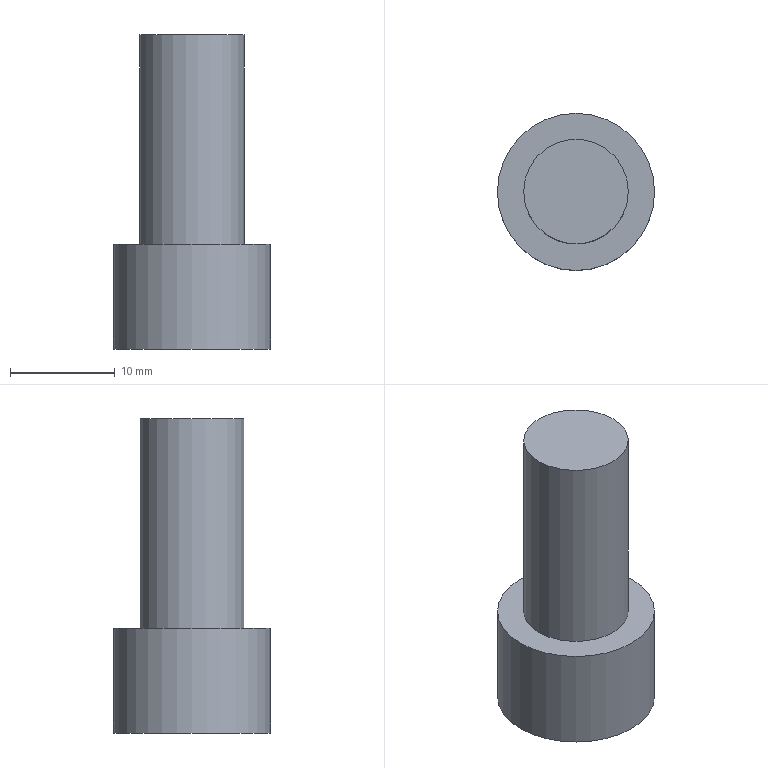Part | NX | features solid 2 | 1 solid | 7 faces | box 15 x 15 x 30 mm | volume 2835 mm3 | plane 4 | cylinder 3 | commonest cylinder face diameters 8 x1 10 x1 15 x1
STEP:
#1=CARTESIAN_POINT('',(-473.,-235.,292.));
#2=VERTEX_POINT('',#1);
#3=CARTESIAN_POINT('',(-478.,-235.,292.));
#4=DIRECTION('',(0.,0.,1.));
#5=DIRECTION('',(1.,0.,0.));
#6=AXIS2_PLACEMENT_3D('',#3,#4,#5);
#7=CIRCLE('',#6,5.);
#8=EDGE_CURVE('',#2,#2,#7,.T.);
#9=ORIENTED_EDGE('',*,*,#8,.F.);
#10=EDGE_LOOP('',(#9));
#11=FACE_BOUND('',#10,.T.);
#12=CARTESIAN_POINT('',(-473.,-235.,272.));
#13=VERTEX_POINT('',#12);
#14=CARTESIAN_POINT('',(-478.,-235.,272.));
#15=DIRECTION('',(0.,0.,1.));
#16=DIRECTION('',(1.,0.,0.));
#17=AXIS2_PLACEMENT_3D('',#14,#15,#16);
#18=CIRCLE('',#17,5.);
#19=EDGE_CURVE('',#13,#13,#18,.T.);
#20=ORIENTED_EDGE('',*,*,#19,.T.);
#21=EDGE_LOOP('',(#20));
#22=FACE_BOUND('',#21,.T.);
#23=CARTESIAN_POINT('',(-478.,-235.,292.));
#24=DIRECTION('',(0.,0.,-1.));
#25=DIRECTION('',(1.,0.,0.));
#26=AXIS2_PLACEMENT_3D('',#23,#24,#25);
#27=CYLINDRICAL_SURFACE('',#26,5.);
#28=ADVANCED_FACE('',(#11,#22),#27,.T.);
#29=ORIENTED_EDGE('',*,*,#8,.T.);
#30=EDGE_LOOP('',(#29));
#31=FACE_BOUND('',#30,.T.);
#32=CARTESIAN_POINT('',(-478.,-235.,292.));
#33=DIRECTION('',(0.,0.,-1.));
#34=DIRECTION('',(1.,0.,0.));
#35=AXIS2_PLACEMENT_3D('',#32,#33,#34);
#36=PLANE('',#35);
#37=ADVANCED_FACE('',(#31),#36,.F.);
#38=CARTESIAN_POINT('',(-470.5,-235.,262.));
#39=VERTEX_POINT('',#38);
#40=CARTESIAN_POINT('',(-478.,-235.,262.));
#41=DIRECTION('',(0.,0.,1.));
#42=DIRECTION('',(1.,0.,0.));
#43=AXIS2_PLACEMENT_3D('',#40,#41,#42);
#44=CIRCLE('',#43,7.5);
#45=EDGE_CURVE('',#39,#39,#44,.T.);
#46=ORIENTED_EDGE('',*,*,#45,.F.);
#47=EDGE_LOOP('',(#46));
#48=FACE_BOUND('',#47,.T.);
#49=CARTESIAN_POINT('',(-474.,-235.,262.));
#50=VERTEX_POINT('',#49);
#51=CARTESIAN_POINT('',(-478.,-235.,262.));
#52=DIRECTION('',(0.,0.,1.));
#53=DIRECTION('',(1.,0.,0.));
#54=AXIS2_PLACEMENT_3D('',#51,#52,#53);
#55=CIRCLE('',#54,4.);
#56=EDGE_CURVE('',#50,#50,#55,.T.);
#57=ORIENTED_EDGE('',*,*,#56,.T.);
#58=EDGE_LOOP('',(#57));
#59=FACE_BOUND('',#58,.T.);
#60=CARTESIAN_POINT('',(-478.,-235.,262.));
#61=DIRECTION('',(0.,0.,1.));
#62=DIRECTION('',(-1.,0.,0.));
#63=AXIS2_PLACEMENT_3D('',#60,#61,#62);
#64=PLANE('',#63);
#65=ADVANCED_FACE('',(#48,#59),#64,.F.);
#66=ORIENTED_EDGE('',*,*,#19,.F.);
#67=EDGE_LOOP('',(#66));
#68=FACE_BOUND('',#67,.T.);
#69=CARTESIAN_POINT('',(-470.5,-235.,272.));
#70=VERTEX_POINT('',#69);
#71=CARTESIAN_POINT('',(-478.,-235.,272.));
#72=DIRECTION('',(0.,0.,1.));
#73=DIRECTION('',(1.,0.,0.));
#74=AXIS2_PLACEMENT_3D('',#71,#72,#73);
#75=CIRCLE('',#74,7.5);
#76=EDGE_CURVE('',#70,#70,#75,.T.);
#77=ORIENTED_EDGE('',*,*,#76,.T.);
#78=EDGE_LOOP('',(#77));
#79=FACE_BOUND('',#78,.T.);
#80=CARTESIAN_POINT('',(-478.,-235.,272.));
#81=DIRECTION('',(0.,0.,1.));
#82=DIRECTION('',(-1.,0.,0.));
#83=AXIS2_PLACEMENT_3D('',#80,#81,#82);
#84=PLANE('',#83);
#85=ADVANCED_FACE('',(#68,#79),#84,.T.);
#86=ORIENTED_EDGE('',*,*,#45,.T.);
#87=EDGE_LOOP('',(#86));
#88=FACE_BOUND('',#87,.T.);
#89=ORIENTED_EDGE('',*,*,#76,.F.);
#90=EDGE_LOOP('',(#89));
#91=FACE_BOUND('',#90,.T.);
#92=CARTESIAN_POINT('',(-478.,-235.,272.));
#93=DIRECTION('',(0.,0.,-1.));
#94=DIRECTION('',(1.,0.,0.));
#95=AXIS2_PLACEMENT_3D('',#92,#93,#94);
#96=CYLINDRICAL_SURFACE('',#95,7.5);
#97=ADVANCED_FACE('',(#88,#91),#96,.T.);
#98=ORIENTED_EDGE('',*,*,#56,.F.);
#99=EDGE_LOOP('',(#98));
#100=FACE_BOUND('',#99,.T.);
#101=CARTESIAN_POINT('',(-474.,-235.,272.));
#102=VERTEX_POINT('',#101);
#103=CARTESIAN_POINT('',(-478.,-235.,272.));
#104=DIRECTION('',(0.,0.,1.));
#105=DIRECTION('',(1.,0.,0.));
#106=AXIS2_PLACEMENT_3D('',#103,#104,#105);
#107=CIRCLE('',#106,4.);
#108=EDGE_CURVE('',#102,#102,#107,.T.);
#109=ORIENTED_EDGE('',*,*,#108,.T.);
#110=EDGE_LOOP('',(#109));
#111=FACE_BOUND('',#110,.T.);
#112=CARTESIAN_POINT('',(-478.,-235.,272.));
#113=DIRECTION('',(0.,0.,-1.));
#114=DIRECTION('',(1.,0.,0.));
#115=AXIS2_PLACEMENT_3D('',#112,#113,#114);
#116=CYLINDRICAL_SURFACE('',#115,4.);
#117=ADVANCED_FACE('',(#100,#111),#116,.F.);
#118=ORIENTED_EDGE('',*,*,#108,.F.);
#119=EDGE_LOOP('',(#118));
#120=FACE_BOUND('',#119,.T.);
#121=CARTESIAN_POINT('',(-478.,-235.,272.));
#122=DIRECTION('',(0.,0.,-1.));
#123=DIRECTION('',(1.,0.,0.));
#124=AXIS2_PLACEMENT_3D('',#121,#122,#123);
#125=PLANE('',#124);
#126=ADVANCED_FACE('',(#120),#125,.T.);
#127=CLOSED_SHELL('',(#28,#37,#65,#85,#97,#117,#126));
#128=MANIFOLD_SOLID_BREP('',#127);
#129=(LENGTH_UNIT()NAMED_UNIT(*)SI_UNIT(.MILLI.,.METRE.));
#130=UNCERTAINTY_MEASURE_WITH_UNIT(LENGTH_MEASURE(0.00001),#129,'','');
#131=(NAMED_UNIT(*)PLANE_ANGLE_UNIT()SI_UNIT($,.RADIAN.));
#132=(NAMED_UNIT(*)SI_UNIT($,.STERADIAN.)SOLID_ANGLE_UNIT());
#133=(GEOMETRIC_REPRESENTATION_CONTEXT(3)GLOBAL_UNCERTAINTY_ASSIGNED_CONTEXT((#130))GLOBAL_UNIT_ASSIGNED_CONTEXT((#129,#131,#132))REPRESENTATION_CONTEXT('',''));
#134=ADVANCED_BREP_SHAPE_REPRESENTATION('',(#128),#133);